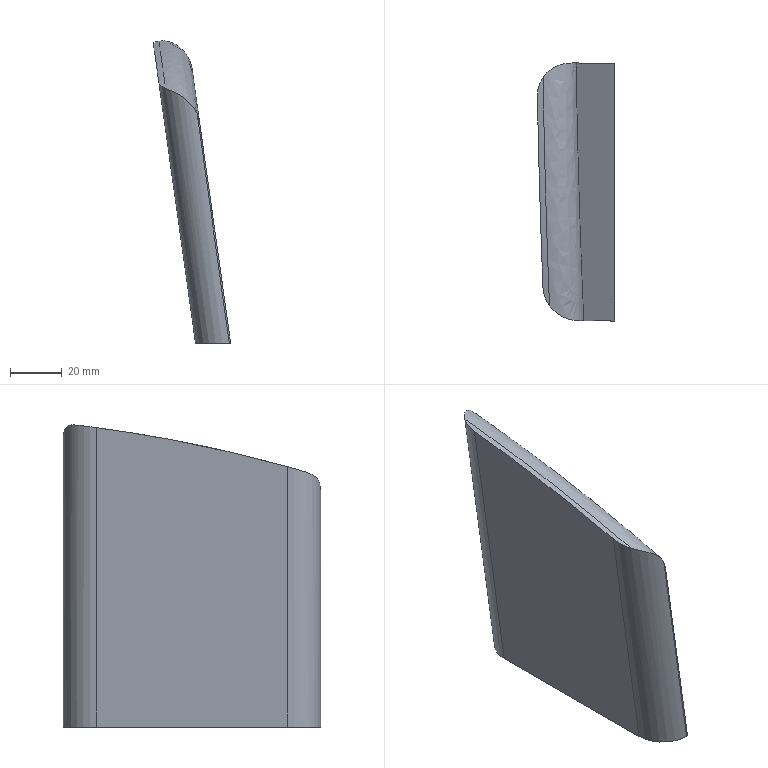Part | STEP file | solid 94 | 1 solid | 9 faces | box 29.965 x 100 x 117.263 mm | volume 138238 mm3 | plane 5 | cylinder 2 | other 1 | spline 1 | commonest cylinder face diameters 26 x2